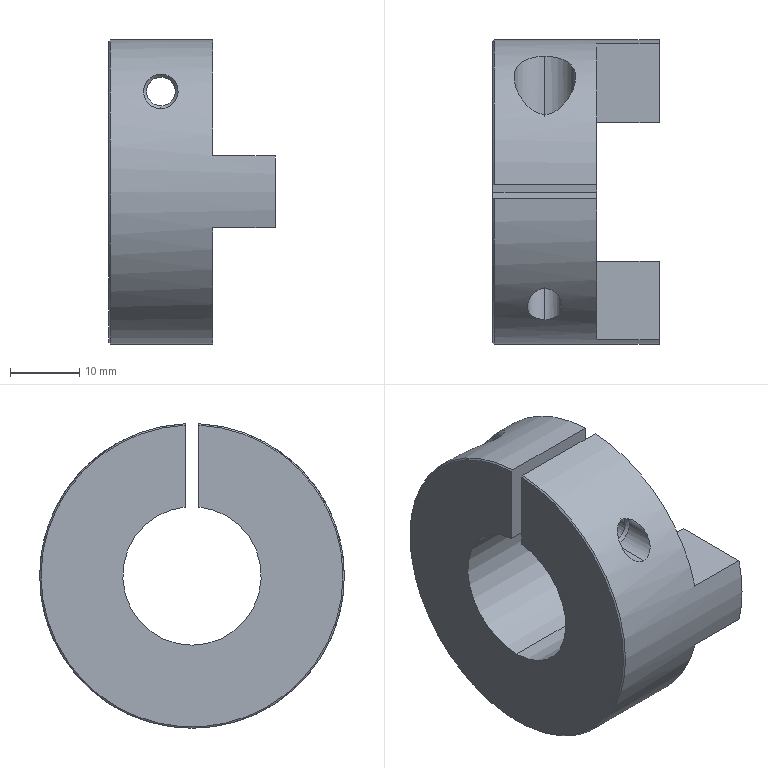Part | STEP file | 0244_Z_008_MFJC44-20-20_2 | 1 solid | 32 faces | box 24 x 44 x 43.977 mm | volume 18858 mm3 | cylinder 14 | plane 11 | cone 7 | commonest cylinder face diameters 5 x4 4.134 x2 8.9 x2 20 x2 22.5 x2 44 x2